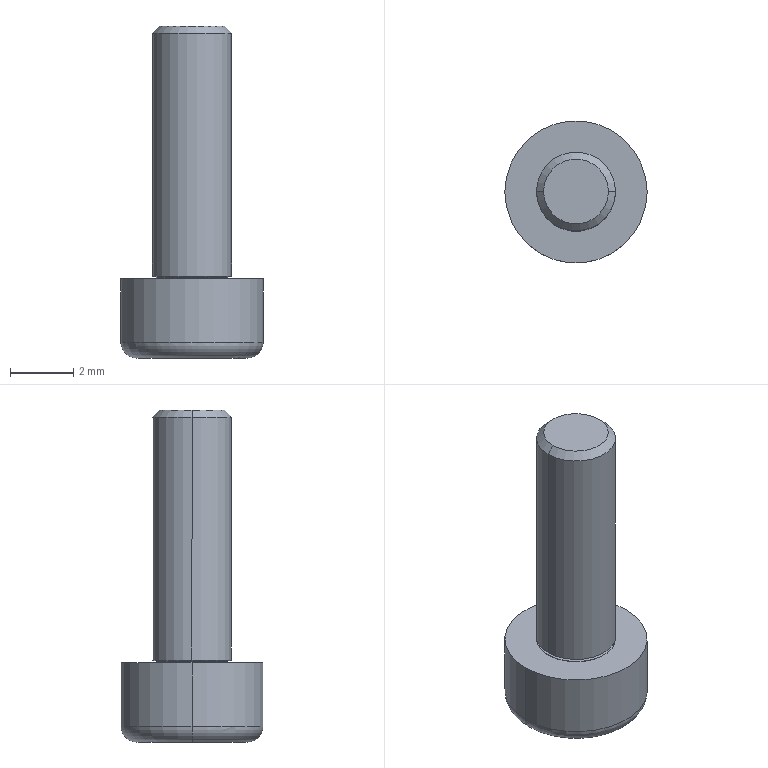Part | SolidWorks | features BaseBody 1 | 1 solid | 27 faces | box 4.5 x 4.5 x 10.5 mm | volume 74.603 mm3 | plane 11 | torus 6 | cylinder 6 | cone 4 | commonest cylinder face diameters 2.5 x4 4.5 x2
STEP:
#1=CARTESIAN_POINT('',(-1.138,0.,0.01));
#2=VERTEX_POINT('',#1);
#3=CARTESIAN_POINT('',(-1.118,0.,0.03));
#4=VERTEX_POINT('',#3);
#5=CARTESIAN_POINT('',(-1.138,0.,0.03));
#6=DIRECTION('',(0.,-1.,0.));
#7=DIRECTION('',(0.,0.,-1.));
#8=AXIS2_PLACEMENT_3D('',#5,#6,#7);
#9=CIRCLE('',#8,0.02);
#10=EDGE_CURVE('',#2,#4,#9,.T.);
#11=ORIENTED_EDGE('',*,*,#10,.T.);
#12=CARTESIAN_POINT('',(1.118,0.,0.03));
#13=VERTEX_POINT('',#12);
#14=CARTESIAN_POINT('',(0.,0.,0.03));
#15=DIRECTION('',(0.,0.,-1.));
#16=DIRECTION('',(-1.,0.,0.));
#17=AXIS2_PLACEMENT_3D('',#14,#15,#16);
#18=CIRCLE('',#17,1.118);
#19=EDGE_CURVE('',#4,#13,#18,.T.);
#20=ORIENTED_EDGE('',*,*,#19,.T.);
#21=CARTESIAN_POINT('',(1.138,0.,0.01));
#22=VERTEX_POINT('',#21);
#23=CARTESIAN_POINT('',(1.138,0.,0.03));
#24=DIRECTION('',(0.,1.,0.));
#25=DIRECTION('',(-1.,0.,0.));
#26=AXIS2_PLACEMENT_3D('',#23,#24,#25);
#27=CIRCLE('',#26,0.02);
#28=EDGE_CURVE('',#22,#13,#27,.T.);
#29=ORIENTED_EDGE('',*,*,#28,.F.);
#30=CARTESIAN_POINT('',(0.,0.,0.01));
#31=DIRECTION('',(0.,0.,-1.));
#32=DIRECTION('',(-1.,0.,0.));
#33=AXIS2_PLACEMENT_3D('',#30,#31,#32);
#34=CIRCLE('',#33,1.138);
#35=EDGE_CURVE('',#2,#22,#34,.T.);
#36=ORIENTED_EDGE('',*,*,#35,.F.);
#37=EDGE_LOOP('',(#11,#20,#29,#36));
#38=FACE_OUTER_BOUND('',#37,.T.);
#39=CARTESIAN_POINT('',(0.,0.,0.03));
#40=DIRECTION('',(0.,0.,-1.));
#41=DIRECTION('',(-1.,0.,0.));
#42=AXIS2_PLACEMENT_3D('',#39,#40,#41);
#43=TOROIDAL_SURFACE('',#42,1.138,0.02);
#44=ADVANCED_FACE('',(#38),#43,.F.);
#45=ORIENTED_EDGE('',*,*,#28,.T.);
#46=CARTESIAN_POINT('',(0.,0.,0.03));
#47=DIRECTION('',(0.,0.,-1.));
#48=DIRECTION('',(-1.,0.,0.));
#49=AXIS2_PLACEMENT_3D('',#46,#47,#48);
#50=CIRCLE('',#49,1.118);
#51=EDGE_CURVE('',#13,#4,#50,.T.);
#52=ORIENTED_EDGE('',*,*,#51,.T.);
#53=ORIENTED_EDGE('',*,*,#10,.F.);
#54=CARTESIAN_POINT('',(0.,0.,0.01));
#55=DIRECTION('',(0.,0.,-1.));
#56=DIRECTION('',(-1.,0.,0.));
#57=AXIS2_PLACEMENT_3D('',#54,#55,#56);
#58=CIRCLE('',#57,1.138);
#59=EDGE_CURVE('',#22,#2,#58,.T.);
#60=ORIENTED_EDGE('',*,*,#59,.F.);
#61=EDGE_LOOP('',(#45,#52,#53,#60));
#62=FACE_OUTER_BOUND('',#61,.T.);
#63=CARTESIAN_POINT('',(0.,0.,0.03));
#64=DIRECTION('',(0.,0.,-1.));
#65=DIRECTION('',(-1.,0.,0.));
#66=AXIS2_PLACEMENT_3D('',#63,#64,#65);
#67=TOROIDAL_SURFACE('',#66,1.138,0.02);
#68=ADVANCED_FACE('',(#62),#67,.F.);
#69=CARTESIAN_POINT('',(-1.025,0.,8.));
#70=VERTEX_POINT('',#69);
#71=CARTESIAN_POINT('',(1.025,0.,8.));
#72=VERTEX_POINT('',#71);
#73=CARTESIAN_POINT('',(0.,0.,8.));
#74=DIRECTION('',(0.,0.,-1.));
#75=DIRECTION('',(-1.,0.,0.));
#76=AXIS2_PLACEMENT_3D('',#73,#74,#75);
#77=CIRCLE('',#76,1.025);
#78=EDGE_CURVE('',#70,#72,#77,.T.);
#79=ORIENTED_EDGE('',*,*,#78,.T.);
#80=CARTESIAN_POINT('',(1.25,0.,7.775));
#81=VERTEX_POINT('',#80);
#82=CARTESIAN_POINT('',(1.025,0.,8.));
#83=DIRECTION('',(0.7071,0.,-0.7071));
#84=VECTOR('',#83,1000.);
#85=LINE('',#82,#84);
#86=EDGE_CURVE('',#72,#81,#85,.T.);
#87=ORIENTED_EDGE('',*,*,#86,.T.);
#88=CARTESIAN_POINT('',(-1.25,0.,7.775));
#89=VERTEX_POINT('',#88);
#90=CARTESIAN_POINT('',(0.,0.,7.775));
#91=DIRECTION('',(0.,0.,-1.));
#92=DIRECTION('',(-1.,0.,0.));
#93=AXIS2_PLACEMENT_3D('',#90,#91,#92);
#94=CIRCLE('',#93,1.25);
#95=EDGE_CURVE('',#89,#81,#94,.T.);
#96=ORIENTED_EDGE('',*,*,#95,.F.);
#97=CARTESIAN_POINT('',(-1.025,0.,8.));
#98=DIRECTION('',(-0.7071,0.,-0.7071));
#99=VECTOR('',#98,1000.);
#100=LINE('',#97,#99);
#101=EDGE_CURVE('',#70,#89,#100,.T.);
#102=ORIENTED_EDGE('',*,*,#101,.F.);
#103=EDGE_LOOP('',(#79,#87,#96,#102));
#104=FACE_OUTER_BOUND('',#103,.T.);
#105=CARTESIAN_POINT('',(0.,0.,8.));
#106=DIRECTION('',(0.,0.,-1.));
#107=DIRECTION('',(-1.,0.,0.));
#108=AXIS2_PLACEMENT_3D('',#105,#106,#107);
#109=CONICAL_SURFACE('',#108,1.025,0.7854);
#110=ADVANCED_FACE('',(#104),#109,.T.);
#111=ORIENTED_EDGE('',*,*,#95,.T.);
#112=CARTESIAN_POINT('',(1.25,0.,0.09189));
#113=VERTEX_POINT('',#112);
#114=CARTESIAN_POINT('',(1.25,0.,-10.585));
#115=DIRECTION('',(0.,0.,-1.));
#116=VECTOR('',#115,1000.);
#117=LINE('',#114,#116);
#118=EDGE_CURVE('',#81,#113,#117,.T.);
#119=ORIENTED_EDGE('',*,*,#118,.T.);
#120=CARTESIAN_POINT('',(-1.25,0.,0.09189));
#121=VERTEX_POINT('',#120);
#122=CARTESIAN_POINT('',(0.,0.,0.09189));
#123=DIRECTION('',(0.,0.,-1.));
#124=DIRECTION('',(-1.,0.,0.));
#125=AXIS2_PLACEMENT_3D('',#122,#123,#124);
#126=CIRCLE('',#125,1.25);
#127=EDGE_CURVE('',#121,#113,#126,.T.);
#128=ORIENTED_EDGE('',*,*,#127,.F.);
#129=CARTESIAN_POINT('',(-1.25,0.,-10.585));
#130=DIRECTION('',(0.,0.,-1.));
#131=VECTOR('',#130,1000.);
#132=LINE('',#129,#131);
#133=EDGE_CURVE('',#89,#121,#132,.T.);
#134=ORIENTED_EDGE('',*,*,#133,.F.);
#135=EDGE_LOOP('',(#111,#119,#128,#134));
#136=FACE_OUTER_BOUND('',#135,.T.);
#137=CARTESIAN_POINT('',(0.,0.,-10.585));
#138=DIRECTION('',(0.,0.,-1.));
#139=DIRECTION('',(-1.,0.,0.));
#140=AXIS2_PLACEMENT_3D('',#137,#138,#139);
#141=CYLINDRICAL_SURFACE('',#140,1.25);
#142=ADVANCED_FACE('',(#136),#141,.T.);
#143=CARTESIAN_POINT('',(-1.132,0.,0.04879));
#144=VERTEX_POINT('',#143);
#145=CARTESIAN_POINT('',(1.132,0.,0.04879));
#146=VERTEX_POINT('',#145);
#147=CARTESIAN_POINT('',(0.,0.,0.04879));
#148=DIRECTION('',(0.,0.,-1.));
#149=DIRECTION('',(-1.,0.,0.));
#150=AXIS2_PLACEMENT_3D('',#147,#148,#149);
#151=CIRCLE('',#150,1.132);
#152=EDGE_CURVE('',#144,#146,#151,.T.);
#153=ORIENTED_EDGE('',*,*,#152,.F.);
#154=CARTESIAN_POINT('',(-1.25,0.,0.09189));
#155=DIRECTION('',(-0.9397,0.,0.342));
#156=VECTOR('',#155,1000.);
#157=LINE('',#154,#156);
#158=EDGE_CURVE('',#144,#121,#157,.T.);
#159=ORIENTED_EDGE('',*,*,#158,.T.);
#160=ORIENTED_EDGE('',*,*,#127,.T.);
#161=CARTESIAN_POINT('',(1.25,0.,0.09189));
#162=DIRECTION('',(0.9397,0.,0.342));
#163=VECTOR('',#162,1000.);
#164=LINE('',#161,#163);
#165=EDGE_CURVE('',#146,#113,#164,.T.);
#166=ORIENTED_EDGE('',*,*,#165,.F.);
#167=EDGE_LOOP('',(#153,#159,#160,#166));
#168=FACE_OUTER_BOUND('',#167,.T.);
#169=CARTESIAN_POINT('',(0.,0.,0.09189));
#170=DIRECTION('',(0.,0.,1.));
#171=DIRECTION('',(1.,0.,0.));
#172=AXIS2_PLACEMENT_3D('',#169,#170,#171);
#173=CONICAL_SURFACE('',#172,1.25,1.222);
#174=ADVANCED_FACE('',(#168),#173,.T.);
#175=ORIENTED_EDGE('',*,*,#51,.F.);
#176=CARTESIAN_POINT('',(1.138,0.,0.03));
#177=DIRECTION('',(0.,1.,0.));
#178=DIRECTION('',(-1.,0.,0.));
#179=AXIS2_PLACEMENT_3D('',#176,#177,#178);
#180=CIRCLE('',#179,0.02);
#181=EDGE_CURVE('',#13,#146,#180,.T.);
#182=ORIENTED_EDGE('',*,*,#181,.T.);
#183=CARTESIAN_POINT('',(0.,0.,0.04879));
#184=DIRECTION('',(0.,0.,-1.));
#185=DIRECTION('',(-1.,0.,0.));
#186=AXIS2_PLACEMENT_3D('',#183,#184,#185);
#187=CIRCLE('',#186,1.132);
#188=EDGE_CURVE('',#146,#144,#187,.T.);
#189=ORIENTED_EDGE('',*,*,#188,.T.);
#190=CARTESIAN_POINT('',(-1.138,0.,0.03));
#191=DIRECTION('',(0.,-1.,0.));
#192=DIRECTION('',(0.,0.,-1.));
#193=AXIS2_PLACEMENT_3D('',#190,#191,#192);
#194=CIRCLE('',#193,0.02);
#195=EDGE_CURVE('',#4,#144,#194,.T.);
#196=ORIENTED_EDGE('',*,*,#195,.F.);
#197=EDGE_LOOP('',(#175,#182,#189,#196));
#198=FACE_OUTER_BOUND('',#197,.T.);
#199=CARTESIAN_POINT('',(0.,0.,0.03));
#200=DIRECTION('',(0.,0.,-1.));
#201=DIRECTION('',(-1.,0.,0.));
#202=AXIS2_PLACEMENT_3D('',#199,#200,#201);
#203=TOROIDAL_SURFACE('',#202,1.138,0.02);
#204=ADVANCED_FACE('',(#198),#203,.F.);
#205=CARTESIAN_POINT('',(-1.25,0.,0.01));
#206=VERTEX_POINT('',#205);
#207=CARTESIAN_POINT('',(1.25,0.,0.01));
#208=VERTEX_POINT('',#207);
#209=CARTESIAN_POINT('',(0.,0.,0.01));
#210=DIRECTION('',(0.,0.,-1.));
#211=DIRECTION('',(-1.,0.,0.));
#212=AXIS2_PLACEMENT_3D('',#209,#210,#211);
#213=CIRCLE('',#212,1.25);
#214=EDGE_CURVE('',#206,#208,#213,.T.);
#215=ORIENTED_EDGE('',*,*,#214,.T.);
#216=CARTESIAN_POINT('',(1.25,0.,0.));
#217=VERTEX_POINT('',#216);
#218=CARTESIAN_POINT('',(1.25,0.,-10.585));
#219=DIRECTION('',(0.,0.,-1.));
#220=VECTOR('',#219,1000.);
#221=LINE('',#218,#220);
#222=EDGE_CURVE('',#208,#217,#221,.T.);
#223=ORIENTED_EDGE('',*,*,#222,.T.);
#224=CARTESIAN_POINT('',(-1.25,0.,0.));
#225=VERTEX_POINT('',#224);
#226=CARTESIAN_POINT('',(0.,0.,0.));
#227=DIRECTION('',(0.,0.,-1.));
#228=DIRECTION('',(-1.,0.,0.));
#229=AXIS2_PLACEMENT_3D('',#226,#227,#228);
#230=CIRCLE('',#229,1.25);
#231=EDGE_CURVE('',#225,#217,#230,.T.);
#232=ORIENTED_EDGE('',*,*,#231,.F.);
#233=CARTESIAN_POINT('',(-1.25,0.,-10.585));
#234=DIRECTION('',(0.,0.,-1.));
#235=VECTOR('',#234,1000.);
#236=LINE('',#233,#235);
#237=EDGE_CURVE('',#206,#225,#236,.T.);
#238=ORIENTED_EDGE('',*,*,#237,.F.);
#239=EDGE_LOOP('',(#215,#223,#232,#238));
#240=FACE_OUTER_BOUND('',#239,.T.);
#241=CARTESIAN_POINT('',(0.,0.,-10.585));
#242=DIRECTION('',(0.,0.,-1.));
#243=DIRECTION('',(-1.,0.,0.));
#244=AXIS2_PLACEMENT_3D('',#241,#242,#243);
#245=CYLINDRICAL_SURFACE('',#244,1.25);
#246=ADVANCED_FACE('',(#240),#245,.T.);
#247=CARTESIAN_POINT('',(-2.25,0.,0.));
#248=VERTEX_POINT('',#247);
#249=CARTESIAN_POINT('',(2.25,0.,0.));
#250=VERTEX_POINT('',#249);
#251=CARTESIAN_POINT('',(0.,0.,0.));
#252=DIRECTION('',(0.,0.,-1.));
#253=DIRECTION('',(-1.,0.,0.));
#254=AXIS2_PLACEMENT_3D('',#251,#252,#253);
#255=CIRCLE('',#254,2.25);
#256=EDGE_CURVE('',#248,#250,#255,.T.);
#257=ORIENTED_EDGE('',*,*,#256,.T.);
#258=CARTESIAN_POINT('',(2.25,0.,-2.));
#259=VERTEX_POINT('',#258);
#260=CARTESIAN_POINT('',(2.25,0.,-10.585));
#261=DIRECTION('',(0.,0.,-1.));
#262=VECTOR('',#261,1000.);
#263=LINE('',#260,#262);
#264=EDGE_CURVE('',#250,#259,#263,.T.);
#265=ORIENTED_EDGE('',*,*,#264,.T.);
#266=CARTESIAN_POINT('',(-2.25,0.,-2.));
#267=VERTEX_POINT('',#266);
#268=CARTESIAN_POINT('',(0.,0.,-2.));
#269=DIRECTION('',(0.,0.,-1.));
#270=DIRECTION('',(-1.,0.,0.));
#271=AXIS2_PLACEMENT_3D('',#268,#269,#270);
#272=CIRCLE('',#271,2.25);
#273=EDGE_CURVE('',#267,#259,#272,.T.);
#274=ORIENTED_EDGE('',*,*,#273,.F.);
#275=CARTESIAN_POINT('',(-2.25,0.,-10.585));
#276=DIRECTION('',(0.,0.,-1.));
#277=VECTOR('',#276,1000.);
#278=LINE('',#275,#277);
#279=EDGE_CURVE('',#248,#267,#278,.T.);
#280=ORIENTED_EDGE('',*,*,#279,.F.);
#281=EDGE_LOOP('',(#257,#265,#274,#280));
#282=FACE_OUTER_BOUND('',#281,.T.);
#283=CARTESIAN_POINT('',(0.,0.,-10.585));
#284=DIRECTION('',(0.,0.,-1.));
#285=DIRECTION('',(-1.,0.,0.));
#286=AXIS2_PLACEMENT_3D('',#283,#284,#285);
#287=CYLINDRICAL_SURFACE('',#286,2.25);
#288=ADVANCED_FACE('',(#282),#287,.T.);
#289=ORIENTED_EDGE('',*,*,#273,.T.);
#290=CARTESIAN_POINT('',(1.75,0.,-2.5));
#291=VERTEX_POINT('',#290);
#292=CARTESIAN_POINT('',(1.75,0.,-2.));
#293=DIRECTION('',(0.,1.,0.));
#294=DIRECTION('',(-1.,0.,0.));
#295=AXIS2_PLACEMENT_3D('',#292,#293,#294);
#296=CIRCLE('',#295,0.5);
#297=EDGE_CURVE('',#259,#291,#296,.T.);
#298=ORIENTED_EDGE('',*,*,#297,.T.);
#299=CARTESIAN_POINT('',(-1.75,0.,-2.5));
#300=VERTEX_POINT('',#299);
#301=CARTESIAN_POINT('',(0.,0.,-2.5));
#302=DIRECTION('',(0.,0.,-1.));
#303=DIRECTION('',(-1.,0.,0.));
#304=AXIS2_PLACEMENT_3D('',#301,#302,#303);
#305=CIRCLE('',#304,1.75);
#306=EDGE_CURVE('',#300,#291,#305,.T.);
#307=ORIENTED_EDGE('',*,*,#306,.F.);
#308=CARTESIAN_POINT('',(-1.75,0.,-2.));
#309=DIRECTION('',(0.,-1.,0.));
#310=DIRECTION('',(0.,0.,-1.));
#311=AXIS2_PLACEMENT_3D('',#308,#309,#310);
#312=CIRCLE('',#311,0.5);
#313=EDGE_CURVE('',#267,#300,#312,.T.);
#314=ORIENTED_EDGE('',*,*,#313,.F.);
#315=EDGE_LOOP('',(#289,#298,#307,#314));
#316=FACE_OUTER_BOUND('',#315,.T.);
#317=CARTESIAN_POINT('',(0.,0.,-2.));
#318=DIRECTION('',(0.,0.,-1.));
#319=DIRECTION('',(-1.,0.,0.));
#320=AXIS2_PLACEMENT_3D('',#317,#318,#319);
#321=TOROIDAL_SURFACE('',#320,1.75,0.5);
#322=ADVANCED_FACE('',(#316),#321,.T.);
#323=ORIENTED_EDGE('',*,*,#297,.F.);
#324=CARTESIAN_POINT('',(0.,0.,-2.));
#325=DIRECTION('',(0.,0.,-1.));
#326=DIRECTION('',(-1.,0.,0.));
#327=AXIS2_PLACEMENT_3D('',#324,#325,#326);
#328=CIRCLE('',#327,2.25);
#329=EDGE_CURVE('',#259,#267,#328,.T.);
#330=ORIENTED_EDGE('',*,*,#329,.T.);
#331=ORIENTED_EDGE('',*,*,#313,.T.);
#332=CARTESIAN_POINT('',(0.,0.,-2.5));
#333=DIRECTION('',(0.,0.,-1.));
#334=DIRECTION('',(-1.,0.,0.));
#335=AXIS2_PLACEMENT_3D('',#332,#333,#334);
#336=CIRCLE('',#335,1.75);
#337=EDGE_CURVE('',#291,#300,#336,.T.);
#338=ORIENTED_EDGE('',*,*,#337,.F.);
#339=EDGE_LOOP('',(#323,#330,#331,#338));
#340=FACE_OUTER_BOUND('',#339,.T.);
#341=CARTESIAN_POINT('',(0.,0.,-2.));
#342=DIRECTION('',(0.,0.,-1.));
#343=DIRECTION('',(-1.,0.,0.));
#344=AXIS2_PLACEMENT_3D('',#341,#342,#343);
#345=TOROIDAL_SURFACE('',#344,1.75,0.5);
#346=ADVANCED_FACE('',(#340),#345,.T.);
#347=ORIENTED_EDGE('',*,*,#264,.F.);
#348=CARTESIAN_POINT('',(0.,0.,0.));
#349=DIRECTION('',(0.,0.,-1.));
#350=DIRECTION('',(-1.,0.,0.));
#351=AXIS2_PLACEMENT_3D('',#348,#349,#350);
#352=CIRCLE('',#351,2.25);
#353=EDGE_CURVE('',#250,#248,#352,.T.);
#354=ORIENTED_EDGE('',*,*,#353,.T.);
#355=ORIENTED_EDGE('',*,*,#279,.T.);
#356=ORIENTED_EDGE('',*,*,#329,.F.);
#357=EDGE_LOOP('',(#347,#354,#355,#356));
#358=FACE_OUTER_BOUND('',#357,.T.);
#359=CARTESIAN_POINT('',(0.,0.,-10.585));
#360=DIRECTION('',(0.,0.,-1.));
#361=DIRECTION('',(-1.,0.,0.));
#362=AXIS2_PLACEMENT_3D('',#359,#360,#361);
#363=CYLINDRICAL_SURFACE('',#362,2.25);
#364=ADVANCED_FACE('',(#358),#363,.T.);
#365=ORIENTED_EDGE('',*,*,#256,.F.);
#366=ORIENTED_EDGE('',*,*,#353,.F.);
#367=EDGE_LOOP('',(#365,#366));
#368=FACE_OUTER_BOUND('',#367,.T.);
#369=ORIENTED_EDGE('',*,*,#231,.T.);
#370=CARTESIAN_POINT('',(0.,0.,0.));
#371=DIRECTION('',(0.,0.,-1.));
#372=DIRECTION('',(-1.,0.,0.));
#373=AXIS2_PLACEMENT_3D('',#370,#371,#372);
#374=CIRCLE('',#373,1.25);
#375=EDGE_CURVE('',#217,#225,#374,.T.);
#376=ORIENTED_EDGE('',*,*,#375,.T.);
#377=EDGE_LOOP('',(#369,#376));
#378=FACE_BOUND('',#377,.T.);
#379=CARTESIAN_POINT('',(-2.25,0.,0.));
#380=DIRECTION('',(0.,0.,-1.));
#381=DIRECTION('',(-1.,0.,0.));
#382=AXIS2_PLACEMENT_3D('',#379,#380,#381);
#383=PLANE('',#382);
#384=ADVANCED_FACE('',(#368,#378),#383,.F.);
#385=ORIENTED_EDGE('',*,*,#222,.F.);
#386=CARTESIAN_POINT('',(0.,0.,0.01));
#387=DIRECTION('',(0.,0.,-1.));
#388=DIRECTION('',(-1.,0.,0.));
#389=AXIS2_PLACEMENT_3D('',#386,#387,#388);
#390=CIRCLE('',#389,1.25);
#391=EDGE_CURVE('',#208,#206,#390,.T.);
#392=ORIENTED_EDGE('',*,*,#391,.T.);
#393=ORIENTED_EDGE('',*,*,#237,.T.);
#394=ORIENTED_EDGE('',*,*,#375,.F.);
#395=EDGE_LOOP('',(#385,#392,#393,#394));
#396=FACE_OUTER_BOUND('',#395,.T.);
#397=CARTESIAN_POINT('',(0.,0.,-10.585));
#398=DIRECTION('',(0.,0.,-1.));
#399=DIRECTION('',(-1.,0.,0.));
#400=AXIS2_PLACEMENT_3D('',#397,#398,#399);
#401=CYLINDRICAL_SURFACE('',#400,1.25);
#402=ADVANCED_FACE('',(#396),#401,.T.);
#403=ORIENTED_EDGE('',*,*,#214,.F.);
#404=ORIENTED_EDGE('',*,*,#391,.F.);
#405=EDGE_LOOP('',(#403,#404));
#406=FACE_OUTER_BOUND('',#405,.T.);
#407=ORIENTED_EDGE('',*,*,#35,.T.);
#408=ORIENTED_EDGE('',*,*,#59,.T.);
#409=EDGE_LOOP('',(#407,#408));
#410=FACE_BOUND('',#409,.T.);
#411=CARTESIAN_POINT('',(-1.25,0.,0.01));
#412=DIRECTION('',(0.,0.,-1.));
#413=DIRECTION('',(-1.,0.,0.));
#414=AXIS2_PLACEMENT_3D('',#411,#412,#413);
#415=PLANE('',#414);
#416=ADVANCED_FACE('',(#406,#410),#415,.F.);
#417=ORIENTED_EDGE('',*,*,#19,.F.);
#418=ORIENTED_EDGE('',*,*,#195,.T.);
#419=ORIENTED_EDGE('',*,*,#152,.T.);
#420=ORIENTED_EDGE('',*,*,#181,.F.);
#421=EDGE_LOOP('',(#417,#418,#419,#420));
#422=FACE_OUTER_BOUND('',#421,.T.);
#423=CARTESIAN_POINT('',(0.,0.,0.03));
#424=DIRECTION('',(0.,0.,-1.));
#425=DIRECTION('',(-1.,0.,0.));
#426=AXIS2_PLACEMENT_3D('',#423,#424,#425);
#427=TOROIDAL_SURFACE('',#426,1.138,0.02);
#428=ADVANCED_FACE('',(#422),#427,.F.);
#429=ORIENTED_EDGE('',*,*,#158,.F.);
#430=ORIENTED_EDGE('',*,*,#188,.F.);
#431=ORIENTED_EDGE('',*,*,#165,.T.);
#432=CARTESIAN_POINT('',(0.,0.,0.09189));
#433=DIRECTION('',(0.,0.,-1.));
#434=DIRECTION('',(-1.,0.,0.));
#435=AXIS2_PLACEMENT_3D('',#432,#433,#434);
#436=CIRCLE('',#435,1.25);
#437=EDGE_CURVE('',#113,#121,#436,.T.);
#438=ORIENTED_EDGE('',*,*,#437,.T.);
#439=EDGE_LOOP('',(#429,#430,#431,#438));
#440=FACE_OUTER_BOUND('',#439,.T.);
#441=CARTESIAN_POINT('',(0.,0.,0.09189));
#442=DIRECTION('',(0.,0.,1.));
#443=DIRECTION('',(1.,0.,0.));
#444=AXIS2_PLACEMENT_3D('',#441,#442,#443);
#445=CONICAL_SURFACE('',#444,1.25,1.222);
#446=ADVANCED_FACE('',(#440),#445,.T.);
#447=ORIENTED_EDGE('',*,*,#118,.F.);
#448=CARTESIAN_POINT('',(0.,0.,7.775));
#449=DIRECTION('',(0.,0.,-1.));
#450=DIRECTION('',(-1.,0.,0.));
#451=AXIS2_PLACEMENT_3D('',#448,#449,#450);
#452=CIRCLE('',#451,1.25);
#453=EDGE_CURVE('',#81,#89,#452,.T.);
#454=ORIENTED_EDGE('',*,*,#453,.T.);
#455=ORIENTED_EDGE('',*,*,#133,.T.);
#456=ORIENTED_EDGE('',*,*,#437,.F.);
#457=EDGE_LOOP('',(#447,#454,#455,#456));
#458=FACE_OUTER_BOUND('',#457,.T.);
#459=CARTESIAN_POINT('',(0.,0.,-10.585));
#460=DIRECTION('',(0.,0.,-1.));
#461=DIRECTION('',(-1.,0.,0.));
#462=AXIS2_PLACEMENT_3D('',#459,#460,#461);
#463=CYLINDRICAL_SURFACE('',#462,1.25);
#464=ADVANCED_FACE('',(#458),#463,.T.);
#465=ORIENTED_EDGE('',*,*,#86,.F.);
#466=CARTESIAN_POINT('',(0.,0.,8.));
#467=DIRECTION('',(0.,0.,-1.));
#468=DIRECTION('',(-1.,0.,0.));
#469=AXIS2_PLACEMENT_3D('',#466,#467,#468);
#470=CIRCLE('',#469,1.025);
#471=EDGE_CURVE('',#72,#70,#470,.T.);
#472=ORIENTED_EDGE('',*,*,#471,.T.);
#473=ORIENTED_EDGE('',*,*,#101,.T.);
#474=ORIENTED_EDGE('',*,*,#453,.F.);
#475=EDGE_LOOP('',(#465,#472,#473,#474));
#476=FACE_OUTER_BOUND('',#475,.T.);
#477=CARTESIAN_POINT('',(0.,0.,8.));
#478=DIRECTION('',(0.,0.,-1.));
#479=DIRECTION('',(-1.,0.,0.));
#480=AXIS2_PLACEMENT_3D('',#477,#478,#479);
#481=CONICAL_SURFACE('',#480,1.025,0.7854);
#482=ADVANCED_FACE('',(#476),#481,.T.);
#483=ORIENTED_EDGE('',*,*,#78,.F.);
#484=ORIENTED_EDGE('',*,*,#471,.F.);
#485=EDGE_LOOP('',(#483,#484));
#486=FACE_OUTER_BOUND('',#485,.T.);
#487=CARTESIAN_POINT('',(-1.025,0.,8.));
#488=DIRECTION('',(0.,0.,-1.));
#489=DIRECTION('',(-1.,0.,0.));
#490=AXIS2_PLACEMENT_3D('',#487,#488,#489);
#491=PLANE('',#490);
#492=ADVANCED_FACE('',(#486),#491,.F.);
#493=CARTESIAN_POINT('',(1.155,0.,-2.5));
#494=VERTEX_POINT('',#493);
#495=CARTESIAN_POINT('',(0.5774,-1.,-2.5));
#496=VERTEX_POINT('',#495);
#497=CARTESIAN_POINT('',(1.155,0.,-2.5));
#498=DIRECTION('',(-0.5,-0.866,0.));
#499=VECTOR('',#498,1000.);
#500=LINE('',#497,#499);
#501=EDGE_CURVE('',#494,#496,#500,.T.);
#502=ORIENTED_EDGE('',*,*,#501,.F.);
#503=CARTESIAN_POINT('',(0.5774,1.,-2.5));
#504=VERTEX_POINT('',#503);
#505=CARTESIAN_POINT('',(0.5774,1.,-2.5));
#506=DIRECTION('',(0.5,-0.866,0.));
#507=VECTOR('',#506,1000.);
#508=LINE('',#505,#507);
#509=EDGE_CURVE('',#504,#494,#508,.T.);
#510=ORIENTED_EDGE('',*,*,#509,.F.);
#511=CARTESIAN_POINT('',(-0.5774,1.,-2.5));
#512=VERTEX_POINT('',#511);
#513=CARTESIAN_POINT('',(-0.5774,1.,-2.5));
#514=DIRECTION('',(1.,0.,0.));
#515=VECTOR('',#514,1000.);
#516=LINE('',#513,#515);
#517=EDGE_CURVE('',#512,#504,#516,.T.);
#518=ORIENTED_EDGE('',*,*,#517,.F.);
#519=CARTESIAN_POINT('',(-1.155,0.,-2.5));
#520=VERTEX_POINT('',#519);
#521=CARTESIAN_POINT('',(-1.155,0.,-2.5));
#522=DIRECTION('',(0.5,0.866,0.));
#523=VECTOR('',#522,1000.);
#524=LINE('',#521,#523);
#525=EDGE_CURVE('',#520,#512,#524,.T.);
#526=ORIENTED_EDGE('',*,*,#525,.F.);
#527=CARTESIAN_POINT('',(-0.5774,-1.,-2.5));
#528=VERTEX_POINT('',#527);
#529=CARTESIAN_POINT('',(-0.5774,-1.,-2.5));
#530=DIRECTION('',(-0.5,0.866,0.));
#531=VECTOR('',#530,1000.);
#532=LINE('',#529,#531);
#533=EDGE_CURVE('',#528,#520,#532,.T.);
#534=ORIENTED_EDGE('',*,*,#533,.F.);
#535=CARTESIAN_POINT('',(0.5774,-1.,-2.5));
#536=DIRECTION('',(-1.,0.,0.));
#537=VECTOR('',#536,1000.);
#538=LINE('',#535,#537);
#539=EDGE_CURVE('',#496,#528,#538,.T.);
#540=ORIENTED_EDGE('',*,*,#539,.F.);
#541=EDGE_LOOP('',(#502,#510,#518,#526,#534,#540));
#542=FACE_BOUND('',#541,.T.);
#543=ORIENTED_EDGE('',*,*,#306,.T.);
#544=ORIENTED_EDGE('',*,*,#337,.T.);
#545=EDGE_LOOP('',(#543,#544));
#546=FACE_OUTER_BOUND('',#545,.T.);
#547=CARTESIAN_POINT('',(0.,0.,-2.5));
#548=DIRECTION('',(0.,0.,1.));
#549=DIRECTION('',(1.,0.,0.));
#550=AXIS2_PLACEMENT_3D('',#547,#548,#549);
#551=PLANE('',#550);
#552=ADVANCED_FACE('',(#542,#546),#551,.F.);
#553=ORIENTED_EDGE('',*,*,#509,.T.);
#554=CARTESIAN_POINT('',(1.155,0.,-1.5));
#555=VERTEX_POINT('',#554);
#556=CARTESIAN_POINT('',(1.155,0.,-1.5));
#557=DIRECTION('',(0.,0.,-1.));
#558=VECTOR('',#557,1000.);
#559=LINE('',#556,#558);
#560=EDGE_CURVE('',#555,#494,#559,.T.);
#561=ORIENTED_EDGE('',*,*,#560,.F.);
#562=CARTESIAN_POINT('',(0.5774,1.,-1.5));
#563=VERTEX_POINT('',#562);
#564=CARTESIAN_POINT('',(0.5774,1.,-1.5));
#565=DIRECTION('',(0.5,-0.866,0.));
#566=VECTOR('',#565,1000.);
#567=LINE('',#564,#566);
#568=EDGE_CURVE('',#563,#555,#567,.T.);
#569=ORIENTED_EDGE('',*,*,#568,.F.);
#570=CARTESIAN_POINT('',(0.5774,1.,-1.5));
#571=DIRECTION('',(0.,0.,-1.));
#572=VECTOR('',#571,1000.);
#573=LINE('',#570,#572);
#574=EDGE_CURVE('',#563,#504,#573,.T.);
#575=ORIENTED_EDGE('',*,*,#574,.T.);
#576=EDGE_LOOP('',(#553,#561,#569,#575));
#577=FACE_OUTER_BOUND('',#576,.T.);
#578=CARTESIAN_POINT('',(0.5774,1.,-1.5));
#579=DIRECTION('',(0.866,0.5,0.));
#580=DIRECTION('',(-0.5,0.866,0.));
#581=AXIS2_PLACEMENT_3D('',#578,#579,#580);
#582=PLANE('',#581);
#583=ADVANCED_FACE('',(#577),#582,.F.);
#584=ORIENTED_EDGE('',*,*,#517,.T.);
#585=ORIENTED_EDGE('',*,*,#574,.F.);
#586=CARTESIAN_POINT('',(-0.5774,1.,-1.5));
#587=VERTEX_POINT('',#586);
#588=CARTESIAN_POINT('',(-0.5774,1.,-1.5));
#589=DIRECTION('',(1.,0.,0.));
#590=VECTOR('',#589,1000.);
#591=LINE('',#588,#590);
#592=EDGE_CURVE('',#587,#563,#591,.T.);
#593=ORIENTED_EDGE('',*,*,#592,.F.);
#594=CARTESIAN_POINT('',(-0.5774,1.,-1.5));
#595=DIRECTION('',(0.,0.,-1.));
#596=VECTOR('',#595,1000.);
#597=LINE('',#594,#596);
#598=EDGE_CURVE('',#587,#512,#597,.T.);
#599=ORIENTED_EDGE('',*,*,#598,.T.);
#600=EDGE_LOOP('',(#584,#585,#593,#599));
#601=FACE_OUTER_BOUND('',#600,.T.);
#602=CARTESIAN_POINT('',(-0.5774,1.,-1.5));
#603=DIRECTION('',(0.,1.,0.));
#604=DIRECTION('',(0.,0.,1.));
#605=AXIS2_PLACEMENT_3D('',#602,#603,#604);
#606=PLANE('',#605);
#607=ADVANCED_FACE('',(#601),#606,.F.);
#608=ORIENTED_EDGE('',*,*,#525,.T.);
#609=ORIENTED_EDGE('',*,*,#598,.F.);
#610=CARTESIAN_POINT('',(-1.155,0.,-1.5));
#611=VERTEX_POINT('',#610);
#612=CARTESIAN_POINT('',(-1.155,0.,-1.5));
#613=DIRECTION('',(0.5,0.866,0.));
#614=VECTOR('',#613,1000.);
#615=LINE('',#612,#614);
#616=EDGE_CURVE('',#611,#587,#615,.T.);
#617=ORIENTED_EDGE('',*,*,#616,.F.);
#618=CARTESIAN_POINT('',(-1.155,0.,-1.5));
#619=DIRECTION('',(0.,0.,-1.));
#620=VECTOR('',#619,1000.);
#621=LINE('',#618,#620);
#622=EDGE_CURVE('',#611,#520,#621,.T.);
#623=ORIENTED_EDGE('',*,*,#622,.T.);
#624=EDGE_LOOP('',(#608,#609,#617,#623));
#625=FACE_OUTER_BOUND('',#624,.T.);
#626=CARTESIAN_POINT('',(-1.155,0.,-1.5));
#627=DIRECTION('',(-0.866,0.5,0.));
#628=DIRECTION('',(-0.5,-0.866,0.));
#629=AXIS2_PLACEMENT_3D('',#626,#627,#628);
#630=PLANE('',#629);
#631=ADVANCED_FACE('',(#625),#630,.F.);
#632=ORIENTED_EDGE('',*,*,#533,.T.);
#633=ORIENTED_EDGE('',*,*,#622,.F.);
#634=CARTESIAN_POINT('',(-0.5774,-1.,-1.5));
#635=VERTEX_POINT('',#634);
#636=CARTESIAN_POINT('',(-0.5774,-1.,-1.5));
#637=DIRECTION('',(-0.5,0.866,0.));
#638=VECTOR('',#637,1000.);
#639=LINE('',#636,#638);
#640=EDGE_CURVE('',#635,#611,#639,.T.);
#641=ORIENTED_EDGE('',*,*,#640,.F.);
#642=CARTESIAN_POINT('',(-0.5774,-1.,-1.5));
#643=DIRECTION('',(0.,0.,-1.));
#644=VECTOR('',#643,1000.);
#645=LINE('',#642,#644);
#646=EDGE_CURVE('',#635,#528,#645,.T.);
#647=ORIENTED_EDGE('',*,*,#646,.T.);
#648=EDGE_LOOP('',(#632,#633,#641,#647));
#649=FACE_OUTER_BOUND('',#648,.T.);
#650=CARTESIAN_POINT('',(-0.5774,-1.,-1.5));
#651=DIRECTION('',(-0.866,-0.5,0.));
#652=DIRECTION('',(0.5,-0.866,0.));
#653=AXIS2_PLACEMENT_3D('',#650,#651,#652);
#654=PLANE('',#653);
#655=ADVANCED_FACE('',(#649),#654,.F.);
#656=ORIENTED_EDGE('',*,*,#539,.T.);
#657=ORIENTED_EDGE('',*,*,#646,.F.);
#658=CARTESIAN_POINT('',(0.5774,-1.,-1.5));
#659=VERTEX_POINT('',#658);
#660=CARTESIAN_POINT('',(0.5774,-1.,-1.5));
#661=DIRECTION('',(-1.,0.,0.));
#662=VECTOR('',#661,1000.);
#663=LINE('',#660,#662);
#664=EDGE_CURVE('',#659,#635,#663,.T.);
#665=ORIENTED_EDGE('',*,*,#664,.F.);
#666=CARTESIAN_POINT('',(0.5774,-1.,-1.5));
#667=DIRECTION('',(0.,0.,-1.));
#668=VECTOR('',#667,1000.);
#669=LINE('',#666,#668);
#670=EDGE_CURVE('',#659,#496,#669,.T.);
#671=ORIENTED_EDGE('',*,*,#670,.T.);
#672=EDGE_LOOP('',(#656,#657,#665,#671));
#673=FACE_OUTER_BOUND('',#672,.T.);
#674=CARTESIAN_POINT('',(0.5774,-1.,-1.5));
#675=DIRECTION('',(0.,-1.,0.));
#676=DIRECTION('',(1.,0.,0.));
#677=AXIS2_PLACEMENT_3D('',#674,#675,#676);
#678=PLANE('',#677);
#679=ADVANCED_FACE('',(#673),#678,.F.);
#680=ORIENTED_EDGE('',*,*,#501,.T.);
#681=ORIENTED_EDGE('',*,*,#670,.F.);
#682=CARTESIAN_POINT('',(1.155,0.,-1.5));
#683=DIRECTION('',(-0.5,-0.866,0.));
#684=VECTOR('',#683,1000.);
#685=LINE('',#682,#684);
#686=EDGE_CURVE('',#555,#659,#685,.T.);
#687=ORIENTED_EDGE('',*,*,#686,.F.);
#688=ORIENTED_EDGE('',*,*,#560,.T.);
#689=EDGE_LOOP('',(#680,#681,#687,#688));
#690=FACE_OUTER_BOUND('',#689,.T.);
#691=CARTESIAN_POINT('',(1.155,0.,-1.5));
#692=DIRECTION('',(0.866,-0.5,0.));
#693=DIRECTION('',(0.5,0.866,0.));
#694=AXIS2_PLACEMENT_3D('',#691,#692,#693);
#695=PLANE('',#694);
#696=ADVANCED_FACE('',(#690),#695,.F.);
#697=ORIENTED_EDGE('',*,*,#568,.T.);
#698=ORIENTED_EDGE('',*,*,#686,.T.);
#699=ORIENTED_EDGE('',*,*,#664,.T.);
#700=ORIENTED_EDGE('',*,*,#640,.T.);
#701=ORIENTED_EDGE('',*,*,#616,.T.);
#702=ORIENTED_EDGE('',*,*,#592,.T.);
#703=EDGE_LOOP('',(#697,#698,#699,#700,#701,#702));
#704=FACE_OUTER_BOUND('',#703,.T.);
#705=CARTESIAN_POINT('',(0.5774,1.,-1.5));
#706=DIRECTION('',(0.,0.,1.));
#707=DIRECTION('',(1.,0.,0.));
#708=AXIS2_PLACEMENT_3D('',#705,#706,#707);
#709=PLANE('',#708);
#710=ADVANCED_FACE('',(#704),#709,.F.);
#711=CLOSED_SHELL('',(#44,#68,#110,#142,#174,#204,#246,#288,#322,#346,#364,#384,#402,#416,#428,#446,#464,#482,#492,#552,#583,#607,#631,#655,#679,#696,#710));
#712=MANIFOLD_SOLID_BREP('',#711);
#713=CARTESIAN_POINT('',(0.,0.,0.));
#714=DIRECTION('',(0.,0.,1.));
#715=DIRECTION('',(1.,0.,0.));
#716=AXIS2_PLACEMENT_3D('',#713,#714,#715);
#717=(LENGTH_UNIT()NAMED_UNIT(*)SI_UNIT(.MILLI.,.METRE.));
#718=UNCERTAINTY_MEASURE_WITH_UNIT(LENGTH_MEASURE(0.00001),#717,'','');
#719=(NAMED_UNIT(*)PLANE_ANGLE_UNIT()SI_UNIT($,.RADIAN.));
#720=(NAMED_UNIT(*)SI_UNIT($,.STERADIAN.)SOLID_ANGLE_UNIT());
#721=(GEOMETRIC_REPRESENTATION_CONTEXT(3)GLOBAL_UNCERTAINTY_ASSIGNED_CONTEXT((#718))GLOBAL_UNIT_ASSIGNED_CONTEXT((#717,#719,#720))REPRESENTATION_CONTEXT('',''));
#722=ADVANCED_BREP_SHAPE_REPRESENTATION('',(#712,#716),#721);